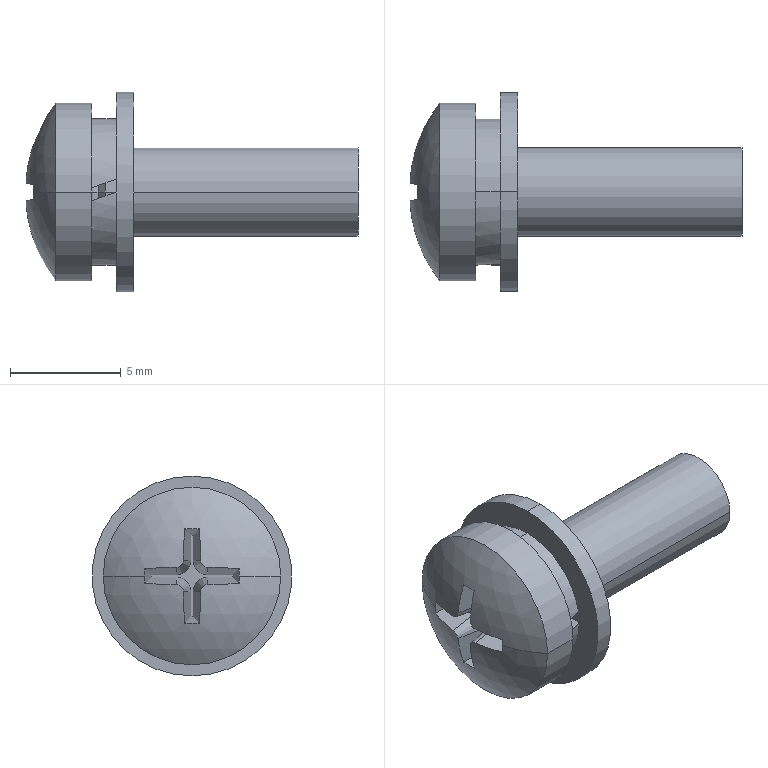Part | SolidWorks | features BaseBody 3 | 3 solids | 45 faces | box 14.964 x 9 x 9 mm | volume 319.965 mm3 | plane 21 | cylinder 14 | cone 6 | sphere 2 | torus 2 | commonest cylinder face diameters 4.4 x3 6.6 x3 4 x2 4.3 x2 8 x2 9 x2
STEP:
#1=CARTESIAN_POINT('',(-133.132,10.87,0.));
#2=VERTEX_POINT('',#1);
#3=CARTESIAN_POINT('',(-133.132,14.87,0.));
#4=VERTEX_POINT('',#3);
#5=CARTESIAN_POINT('',(-133.132,12.87,0.));
#6=DIRECTION('',(-1.,0.,0.));
#7=DIRECTION('',(0.,-1.,0.));
#8=AXIS2_PLACEMENT_3D('',#5,#6,#7);
#9=CIRCLE('',#8,2.);
#10=EDGE_CURVE('',#2,#4,#9,.T.);
#11=ORIENTED_EDGE('',*,*,#10,.T.);
#12=CARTESIAN_POINT('',(-144.532,14.87,0.));
#13=VERTEX_POINT('',#12);
#14=CARTESIAN_POINT('',(-148.132,14.87,0.));
#15=DIRECTION('',(-1.,0.,0.));
#16=VECTOR('',#15,1000.);
#17=LINE('',#14,#16);
#18=EDGE_CURVE('',#4,#13,#17,.T.);
#19=ORIENTED_EDGE('',*,*,#18,.T.);
#20=CARTESIAN_POINT('',(-144.532,10.87,0.));
#21=VERTEX_POINT('',#20);
#22=CARTESIAN_POINT('',(-144.532,12.87,0.));
#23=DIRECTION('',(-1.,0.,0.));
#24=DIRECTION('',(0.,-1.,0.));
#25=AXIS2_PLACEMENT_3D('',#22,#23,#24);
#26=CIRCLE('',#25,2.);
#27=EDGE_CURVE('',#21,#13,#26,.T.);
#28=ORIENTED_EDGE('',*,*,#27,.F.);
#29=CARTESIAN_POINT('',(-148.132,10.87,0.));
#30=DIRECTION('',(-1.,0.,0.));
#31=VECTOR('',#30,1000.);
#32=LINE('',#29,#31);
#33=EDGE_CURVE('',#2,#21,#32,.T.);
#34=ORIENTED_EDGE('',*,*,#33,.F.);
#35=EDGE_LOOP('',(#11,#19,#28,#34));
#36=FACE_OUTER_BOUND('',#35,.T.);
#37=CARTESIAN_POINT('',(-148.132,12.87,0.));
#38=DIRECTION('',(-1.,0.,0.));
#39=DIRECTION('',(0.,-1.,0.));
#40=AXIS2_PLACEMENT_3D('',#37,#38,#39);
#41=CYLINDRICAL_SURFACE('',#40,2.);
#42=ADVANCED_FACE('',(#36),#41,.T.);
#43=CARTESIAN_POINT('',(-146.755,16.87,0.));
#44=VERTEX_POINT('',#43);
#45=CARTESIAN_POINT('',(-146.755,8.87,0.));
#46=VERTEX_POINT('',#45);
#47=CARTESIAN_POINT('',(-146.755,12.87,0.));
#48=DIRECTION('',(-1.,0.,0.));
#49=DIRECTION('',(0.,-1.,0.));
#50=AXIS2_PLACEMENT_3D('',#47,#48,#49);
#51=CIRCLE('',#50,4.);
#52=EDGE_CURVE('',#44,#46,#51,.T.);
#53=ORIENTED_EDGE('',*,*,#52,.T.);
#54=CARTESIAN_POINT('',(-147.771,10.734,0.));
#55=VERTEX_POINT('',#54);
#56=CARTESIAN_POINT('',(-141.632,12.87,0.));
#57=DIRECTION('',(0.,0.,-1.));
#58=DIRECTION('',(0.,1.,0.));
#59=AXIS2_PLACEMENT_3D('',#56,#57,#58);
#60=CIRCLE('',#59,6.5);
#61=EDGE_CURVE('',#46,#55,#60,.T.);
#62=ORIENTED_EDGE('',*,*,#61,.T.);
#63=CARTESIAN_POINT('',(-147.762,10.735,-0.3348));
#64=VERTEX_POINT('',#63);
#65=CARTESIAN_POINT('',(-141.451,11.848,0.));
#66=DIRECTION('',(0.1736,-0.9848,0.));
#67=DIRECTION('',(0.9848,0.1736,0.));
#68=AXIS2_PLACEMENT_3D('',#65,#66,#67);
#69=CIRCLE('',#68,6.417);
#70=EDGE_CURVE('',#55,#64,#69,.T.);
#71=ORIENTED_EDGE('',*,*,#70,.T.);
#72=CARTESIAN_POINT('',(-148.082,12.17,-0.3912));
#73=VERTEX_POINT('',#72);
#74=CARTESIAN_POINT('',(-141.759,12.87,0.7236));
#75=DIRECTION('',(0.1736,0.,-0.9848));
#76=DIRECTION('',(-0.9848,0.,-0.1736));
#77=AXIS2_PLACEMENT_3D('',#74,#75,#76);
#78=CIRCLE('',#77,6.458);
#79=EDGE_CURVE('',#64,#73,#78,.T.);
#80=ORIENTED_EDGE('',*,*,#79,.T.);
#81=CARTESIAN_POINT('',(-148.082,12.479,-0.7));
#82=VERTEX_POINT('',#81);
#83=CARTESIAN_POINT('',(-148.082,12.17,-0.3912));
#84=CARTESIAN_POINT('',(-148.091,12.251,-0.3928));
#85=CARTESIAN_POINT('',(-148.096,12.33,-0.4265));
#86=CARTESIAN_POINT('',(-148.096,12.444,-0.5401));
#87=CARTESIAN_POINT('',(-148.091,12.477,-0.6192));
#88=CARTESIAN_POINT('',(-148.082,12.479,-0.7));
#89=B_SPLINE_CURVE_WITH_KNOTS('',3,(#83,#84,#85,#86,#87,#88),.UNSPECIFIED.,.F.,.F.,(4,2,4),(0.000000198,0.0002406,0.0004811),.UNSPECIFIED.);
#90=EDGE_CURVE('',#73,#82,#89,.T.);
#91=ORIENTED_EDGE('',*,*,#90,.T.);
#92=CARTESIAN_POINT('',(-147.762,12.535,-2.135));
#93=VERTEX_POINT('',#92);
#94=CARTESIAN_POINT('',(-141.759,13.594,0.));
#95=DIRECTION('',(0.1736,-0.9848,0.));
#96=DIRECTION('',(0.9848,0.1736,0.));
#97=AXIS2_PLACEMENT_3D('',#94,#95,#96);
#98=CIRCLE('',#97,6.458);
#99=EDGE_CURVE('',#82,#93,#98,.T.);
#100=ORIENTED_EDGE('',*,*,#99,.T.);
#101=CARTESIAN_POINT('',(-147.762,13.205,-2.135));
#102=VERTEX_POINT('',#101);
#103=CARTESIAN_POINT('',(-141.451,12.87,-1.022));
#104=DIRECTION('',(0.1736,0.,-0.9848));
#105=DIRECTION('',(-0.9848,0.,-0.1736));
#106=AXIS2_PLACEMENT_3D('',#103,#104,#105);
#107=CIRCLE('',#106,6.417);
#108=EDGE_CURVE('',#93,#102,#107,.T.);
#109=ORIENTED_EDGE('',*,*,#108,.T.);
#110=CARTESIAN_POINT('',(-148.082,13.261,-0.7));
#111=VERTEX_POINT('',#110);
#112=CARTESIAN_POINT('',(-141.759,12.147,0.));
#113=DIRECTION('',(0.1736,0.9848,0.));
#114=DIRECTION('',(-0.9848,0.1736,0.));
#115=AXIS2_PLACEMENT_3D('',#112,#113,#114);
#116=CIRCLE('',#115,6.458);
#117=EDGE_CURVE('',#102,#111,#116,.T.);
#118=ORIENTED_EDGE('',*,*,#117,.T.);
#119=CARTESIAN_POINT('',(-148.082,13.57,-0.3912));
#120=VERTEX_POINT('',#119);
#121=CARTESIAN_POINT('',(-148.082,13.261,-0.7));
#122=CARTESIAN_POINT('',(-148.091,13.263,-0.6192));
#123=CARTESIAN_POINT('',(-148.096,13.297,-0.5403));
#124=CARTESIAN_POINT('',(-148.096,13.41,-0.4266));
#125=CARTESIAN_POINT('',(-148.091,13.489,-0.3928));
#126=CARTESIAN_POINT('',(-148.082,13.57,-0.3912));
#127=B_SPLINE_CURVE_WITH_KNOTS('',3,(#121,#122,#123,#124,#125,#126),.UNSPECIFIED.,.F.,.F.,(4,2,4),(0.000000198,0.0002406,0.0004811),.UNSPECIFIED.);
#128=EDGE_CURVE('',#111,#120,#127,.T.);
#129=ORIENTED_EDGE('',*,*,#128,.T.);
#130=CARTESIAN_POINT('',(-147.762,15.005,-0.3348));
#131=VERTEX_POINT('',#130);
#132=CARTESIAN_POINT('',(-141.759,12.87,0.7236));
#133=DIRECTION('',(0.1736,0.,-0.9848));
#134=DIRECTION('',(-0.9848,0.,-0.1736));
#135=AXIS2_PLACEMENT_3D('',#132,#133,#134);
#136=CIRCLE('',#135,6.458);
#137=EDGE_CURVE('',#120,#131,#136,.T.);
#138=ORIENTED_EDGE('',*,*,#137,.T.);
#139=CARTESIAN_POINT('',(-147.771,15.007,0.));
#140=VERTEX_POINT('',#139);
#141=CARTESIAN_POINT('',(-141.451,13.892,0.));
#142=DIRECTION('',(0.1736,0.9848,0.));
#143=DIRECTION('',(-0.9848,0.1736,0.));
#144=AXIS2_PLACEMENT_3D('',#141,#142,#143);
#145=CIRCLE('',#144,6.417);
#146=EDGE_CURVE('',#131,#140,#145,.T.);
#147=ORIENTED_EDGE('',*,*,#146,.T.);
#148=CARTESIAN_POINT('',(-141.632,12.87,0.));
#149=DIRECTION('',(0.,0.,1.));
#150=DIRECTION('',(1.,0.,0.));
#151=AXIS2_PLACEMENT_3D('',#148,#149,#150);
#152=CIRCLE('',#151,6.5);
#153=EDGE_CURVE('',#44,#140,#152,.T.);
#154=ORIENTED_EDGE('',*,*,#153,.F.);
#155=EDGE_LOOP('',(#53,#62,#71,#80,#91,#100,#109,#118,#129,#138,#147,#154));
#156=FACE_OUTER_BOUND('',#155,.T.);
#157=CARTESIAN_POINT('',(-141.632,12.87,0.));
#158=DIRECTION('',(0.,0.,-1.));
#159=DIRECTION('',(0.,1.,0.));
#160=AXIS2_PLACEMENT_3D('',#157,#158,#159);
#161=SPHERICAL_SURFACE('',#160,6.5);
#162=ADVANCED_FACE('',(#156),#161,.T.);
#163=CARTESIAN_POINT('',(-145.132,8.87,0.));
#164=VERTEX_POINT('',#163);
#165=CARTESIAN_POINT('',(-145.132,16.87,0.));
#166=VERTEX_POINT('',#165);
#167=CARTESIAN_POINT('',(-145.132,12.87,0.));
#168=DIRECTION('',(-1.,0.,0.));
#169=DIRECTION('',(0.,-1.,0.));
#170=AXIS2_PLACEMENT_3D('',#167,#168,#169);
#171=CIRCLE('',#170,4.);
#172=EDGE_CURVE('',#164,#166,#171,.T.);
#173=ORIENTED_EDGE('',*,*,#172,.T.);
#174=CARTESIAN_POINT('',(-148.132,16.87,0.));
#175=DIRECTION('',(-1.,0.,0.));
#176=VECTOR('',#175,1000.);
#177=LINE('',#174,#176);
#178=EDGE_CURVE('',#166,#44,#177,.T.);
#179=ORIENTED_EDGE('',*,*,#178,.T.);
#180=CARTESIAN_POINT('',(-146.755,12.87,0.));
#181=DIRECTION('',(-1.,0.,0.));
#182=DIRECTION('',(0.,-1.,0.));
#183=AXIS2_PLACEMENT_3D('',#180,#181,#182);
#184=CIRCLE('',#183,4.);
#185=EDGE_CURVE('',#46,#44,#184,.T.);
#186=ORIENTED_EDGE('',*,*,#185,.F.);
#187=CARTESIAN_POINT('',(-148.132,8.87,0.));
#188=DIRECTION('',(-1.,0.,0.));
#189=VECTOR('',#188,1000.);
#190=LINE('',#187,#189);
#191=EDGE_CURVE('',#164,#46,#190,.T.);
#192=ORIENTED_EDGE('',*,*,#191,.F.);
#193=EDGE_LOOP('',(#173,#179,#186,#192));
#194=FACE_OUTER_BOUND('',#193,.T.);
#195=CARTESIAN_POINT('',(-148.132,12.87,0.));
#196=DIRECTION('',(-1.,0.,0.));
#197=DIRECTION('',(0.,-1.,0.));
#198=AXIS2_PLACEMENT_3D('',#195,#196,#197);
#199=CYLINDRICAL_SURFACE('',#198,4.);
#200=ADVANCED_FACE('',(#194),#199,.T.);
#201=CARTESIAN_POINT('',(-145.132,14.87,0.));
#202=VERTEX_POINT('',#201);
#203=CARTESIAN_POINT('',(-145.132,10.87,0.));
#204=VERTEX_POINT('',#203);
#205=CARTESIAN_POINT('',(-145.132,12.87,0.));
#206=DIRECTION('',(-1.,0.,0.));
#207=DIRECTION('',(0.,-1.,0.));
#208=AXIS2_PLACEMENT_3D('',#205,#206,#207);
#209=CIRCLE('',#208,2.);
#210=EDGE_CURVE('',#202,#204,#209,.T.);
#211=ORIENTED_EDGE('',*,*,#210,.F.);
#212=CARTESIAN_POINT('',(-144.832,14.57,0.));
#213=VERTEX_POINT('',#212);
#214=CARTESIAN_POINT('',(-144.832,14.87,0.));
#215=DIRECTION('',(0.,0.,1.));
#216=DIRECTION('',(0.,-1.,0.));
#217=AXIS2_PLACEMENT_3D('',#214,#215,#216);
#218=CIRCLE('',#217,0.3);
#219=EDGE_CURVE('',#202,#213,#218,.T.);
#220=ORIENTED_EDGE('',*,*,#219,.T.);
#221=CARTESIAN_POINT('',(-144.832,11.17,0.));
#222=VERTEX_POINT('',#221);
#223=CARTESIAN_POINT('',(-144.832,12.87,0.));
#224=DIRECTION('',(-1.,0.,0.));
#225=DIRECTION('',(0.,-1.,0.));
#226=AXIS2_PLACEMENT_3D('',#223,#224,#225);
#227=CIRCLE('',#226,1.7);
#228=EDGE_CURVE('',#213,#222,#227,.T.);
#229=ORIENTED_EDGE('',*,*,#228,.T.);
#230=CARTESIAN_POINT('',(-144.832,10.87,0.));
#231=DIRECTION('',(0.,0.,-1.));
#232=DIRECTION('',(-1.,0.,0.));
#233=AXIS2_PLACEMENT_3D('',#230,#231,#232);
#234=CIRCLE('',#233,0.3);
#235=EDGE_CURVE('',#204,#222,#234,.T.);
#236=ORIENTED_EDGE('',*,*,#235,.F.);
#237=EDGE_LOOP('',(#211,#220,#229,#236));
#238=FACE_OUTER_BOUND('',#237,.T.);
#239=CARTESIAN_POINT('',(-144.832,12.87,0.));
#240=DIRECTION('',(-1.,0.,0.));
#241=DIRECTION('',(0.,-1.,0.));
#242=AXIS2_PLACEMENT_3D('',#239,#240,#241);
#243=TOROIDAL_SURFACE('',#242,2.,0.3);
#244=ADVANCED_FACE('',(#238),#243,.F.);
#245=CARTESIAN_POINT('',(-144.832,12.87,0.));
#246=DIRECTION('',(-1.,0.,0.));
#247=DIRECTION('',(0.,-1.,0.));
#248=AXIS2_PLACEMENT_3D('',#245,#246,#247);
#249=CIRCLE('',#248,1.7);
#250=EDGE_CURVE('',#222,#213,#249,.T.);
#251=ORIENTED_EDGE('',*,*,#250,.F.);
#252=CARTESIAN_POINT('',(-144.832,11.17,0.));
#253=DIRECTION('',(0.7071,-0.7071,0.));
#254=VECTOR('',#253,1000.);
#255=LINE('',#252,#254);
#256=EDGE_CURVE('',#222,#21,#255,.T.);
#257=ORIENTED_EDGE('',*,*,#256,.T.);
#258=ORIENTED_EDGE('',*,*,#27,.T.);
#259=CARTESIAN_POINT('',(-144.832,14.57,0.));
#260=DIRECTION('',(0.7071,0.7071,0.));
#261=VECTOR('',#260,1000.);
#262=LINE('',#259,#261);
#263=EDGE_CURVE('',#213,#13,#262,.T.);
#264=ORIENTED_EDGE('',*,*,#263,.F.);
#265=EDGE_LOOP('',(#251,#257,#258,#264));
#266=FACE_OUTER_BOUND('',#265,.T.);
#267=CARTESIAN_POINT('',(-144.832,12.87,0.));
#268=DIRECTION('',(1.,0.,0.));
#269=DIRECTION('',(0.,1.,0.));
#270=AXIS2_PLACEMENT_3D('',#267,#268,#269);
#271=CONICAL_SURFACE('',#270,1.7,0.7854);
#272=ADVANCED_FACE('',(#266),#271,.T.);
#273=ORIENTED_EDGE('',*,*,#256,.F.);
#274=ORIENTED_EDGE('',*,*,#228,.F.);
#275=ORIENTED_EDGE('',*,*,#263,.T.);
#276=CARTESIAN_POINT('',(-144.532,12.87,0.));
#277=DIRECTION('',(-1.,0.,0.));
#278=DIRECTION('',(0.,-1.,0.));
#279=AXIS2_PLACEMENT_3D('',#276,#277,#278);
#280=CIRCLE('',#279,2.);
#281=EDGE_CURVE('',#13,#21,#280,.T.);
#282=ORIENTED_EDGE('',*,*,#281,.T.);
#283=EDGE_LOOP('',(#273,#274,#275,#282));
#284=FACE_OUTER_BOUND('',#283,.T.);
#285=CARTESIAN_POINT('',(-144.832,12.87,0.));
#286=DIRECTION('',(1.,0.,0.));
#287=DIRECTION('',(0.,1.,0.));
#288=AXIS2_PLACEMENT_3D('',#285,#286,#287);
#289=CONICAL_SURFACE('',#288,1.7,0.7854);
#290=ADVANCED_FACE('',(#284),#289,.T.);
#291=ORIENTED_EDGE('',*,*,#219,.F.);
#292=CARTESIAN_POINT('',(-145.132,12.87,0.));
#293=DIRECTION('',(-1.,0.,0.));
#294=DIRECTION('',(0.,-1.,0.));
#295=AXIS2_PLACEMENT_3D('',#292,#293,#294);
#296=CIRCLE('',#295,2.);
#297=EDGE_CURVE('',#204,#202,#296,.T.);
#298=ORIENTED_EDGE('',*,*,#297,.F.);
#299=ORIENTED_EDGE('',*,*,#235,.T.);
#300=ORIENTED_EDGE('',*,*,#250,.T.);
#301=EDGE_LOOP('',(#291,#298,#299,#300));
#302=FACE_OUTER_BOUND('',#301,.T.);
#303=CARTESIAN_POINT('',(-144.832,12.87,0.));
#304=DIRECTION('',(-1.,0.,0.));
#305=DIRECTION('',(0.,-1.,0.));
#306=AXIS2_PLACEMENT_3D('',#303,#304,#305);
#307=TOROIDAL_SURFACE('',#306,2.,0.3);
#308=ADVANCED_FACE('',(#302),#307,.F.);
#309=ORIENTED_EDGE('',*,*,#172,.F.);
#310=CARTESIAN_POINT('',(-145.132,12.87,0.));
#311=DIRECTION('',(-1.,0.,0.));
#312=DIRECTION('',(0.,-1.,0.));
#313=AXIS2_PLACEMENT_3D('',#310,#311,#312);
#314=CIRCLE('',#313,4.);
#315=EDGE_CURVE('',#166,#164,#314,.T.);
#316=ORIENTED_EDGE('',*,*,#315,.F.);
#317=EDGE_LOOP('',(#309,#316));
#318=FACE_OUTER_BOUND('',#317,.T.);
#319=ORIENTED_EDGE('',*,*,#297,.T.);
#320=ORIENTED_EDGE('',*,*,#210,.T.);
#321=EDGE_LOOP('',(#319,#320));
#322=FACE_BOUND('',#321,.T.);
#323=CARTESIAN_POINT('',(-145.132,12.87,0.));
#324=DIRECTION('',(-1.,0.,0.));
#325=DIRECTION('',(0.,-1.,0.));
#326=AXIS2_PLACEMENT_3D('',#323,#324,#325);
#327=PLANE('',#326);
#328=ADVANCED_FACE('',(#318,#322),#327,.F.);
#329=ORIENTED_EDGE('',*,*,#178,.F.);
#330=ORIENTED_EDGE('',*,*,#315,.T.);
#331=ORIENTED_EDGE('',*,*,#191,.T.);
#332=ORIENTED_EDGE('',*,*,#52,.F.);
#333=EDGE_LOOP('',(#329,#330,#331,#332));
#334=FACE_OUTER_BOUND('',#333,.T.);
#335=CARTESIAN_POINT('',(-148.132,12.87,0.));
#336=DIRECTION('',(-1.,0.,0.));
#337=DIRECTION('',(0.,-1.,0.));
#338=AXIS2_PLACEMENT_3D('',#335,#336,#337);
#339=CYLINDRICAL_SURFACE('',#338,4.);
#340=ADVANCED_FACE('',(#334),#339,.T.);
#341=ORIENTED_EDGE('',*,*,#61,.F.);
#342=ORIENTED_EDGE('',*,*,#185,.T.);
#343=ORIENTED_EDGE('',*,*,#153,.T.);
#344=CARTESIAN_POINT('',(-147.762,15.005,0.3348));
#345=VERTEX_POINT('',#344);
#346=CARTESIAN_POINT('',(-141.451,13.892,0.));
#347=DIRECTION('',(0.1736,0.9848,0.));
#348=DIRECTION('',(-0.9848,0.1736,0.));
#349=AXIS2_PLACEMENT_3D('',#346,#347,#348);
#350=CIRCLE('',#349,6.417);
#351=EDGE_CURVE('',#140,#345,#350,.T.);
#352=ORIENTED_EDGE('',*,*,#351,.T.);
#353=CARTESIAN_POINT('',(-148.082,13.57,0.3912));
#354=VERTEX_POINT('',#353);
#355=CARTESIAN_POINT('',(-141.759,12.87,-0.7236));
#356=DIRECTION('',(0.1736,0.,0.9848));
#357=DIRECTION('',(0.9848,0.,-0.1736));
#358=AXIS2_PLACEMENT_3D('',#355,#356,#357);
#359=CIRCLE('',#358,6.458);
#360=EDGE_CURVE('',#345,#354,#359,.T.);
#361=ORIENTED_EDGE('',*,*,#360,.T.);
#362=CARTESIAN_POINT('',(-148.082,13.261,0.7));
#363=VERTEX_POINT('',#362);
#364=CARTESIAN_POINT('',(-148.082,13.57,0.3912));
#365=CARTESIAN_POINT('',(-148.091,13.489,0.3928));
#366=CARTESIAN_POINT('',(-148.096,13.41,0.4265));
#367=CARTESIAN_POINT('',(-148.096,13.297,0.5401));
#368=CARTESIAN_POINT('',(-148.091,13.263,0.6192));
#369=CARTESIAN_POINT('',(-148.082,13.261,0.7));
#370=B_SPLINE_CURVE_WITH_KNOTS('',3,(#364,#365,#366,#367,#368,#369),.UNSPECIFIED.,.F.,.F.,(4,2,4),(0.000000198,0.0002406,0.0004811),.UNSPECIFIED.);
#371=EDGE_CURVE('',#354,#363,#370,.T.);
#372=ORIENTED_EDGE('',*,*,#371,.T.);
#373=CARTESIAN_POINT('',(-147.762,13.205,2.135));
#374=VERTEX_POINT('',#373);
#375=CARTESIAN_POINT('',(-141.759,12.147,0.));
#376=DIRECTION('',(0.1736,0.9848,0.));
#377=DIRECTION('',(-0.9848,0.1736,0.));
#378=AXIS2_PLACEMENT_3D('',#375,#376,#377);
#379=CIRCLE('',#378,6.458);
#380=EDGE_CURVE('',#363,#374,#379,.T.);
#381=ORIENTED_EDGE('',*,*,#380,.T.);
#382=CARTESIAN_POINT('',(-147.762,12.535,2.135));
#383=VERTEX_POINT('',#382);
#384=CARTESIAN_POINT('',(-141.451,12.87,1.022));
#385=DIRECTION('',(0.1736,0.,0.9848));
#386=DIRECTION('',(0.9848,0.,-0.1736));
#387=AXIS2_PLACEMENT_3D('',#384,#385,#386);
#388=CIRCLE('',#387,6.417);
#389=EDGE_CURVE('',#374,#383,#388,.T.);
#390=ORIENTED_EDGE('',*,*,#389,.T.);
#391=CARTESIAN_POINT('',(-148.082,12.479,0.7));
#392=VERTEX_POINT('',#391);
#393=CARTESIAN_POINT('',(-141.759,13.594,0.));
#394=DIRECTION('',(0.1736,-0.9848,0.));
#395=DIRECTION('',(0.9848,0.1736,0.));
#396=AXIS2_PLACEMENT_3D('',#393,#394,#395);
#397=CIRCLE('',#396,6.458);
#398=EDGE_CURVE('',#383,#392,#397,.T.);
#399=ORIENTED_EDGE('',*,*,#398,.T.);
#400=CARTESIAN_POINT('',(-148.082,12.17,0.3912));
#401=VERTEX_POINT('',#400);
#402=CARTESIAN_POINT('',(-148.082,12.479,0.7));
#403=CARTESIAN_POINT('',(-148.091,12.477,0.6192));
#404=CARTESIAN_POINT('',(-148.096,12.444,0.5403));
#405=CARTESIAN_POINT('',(-148.096,12.33,0.4266));
#406=CARTESIAN_POINT('',(-148.091,12.251,0.3928));
#407=CARTESIAN_POINT('',(-148.082,12.17,0.3912));
#408=B_SPLINE_CURVE_WITH_KNOTS('',3,(#402,#403,#404,#405,#406,#407),.UNSPECIFIED.,.F.,.F.,(4,2,4),(0.000000198,0.0002406,0.0004811),.UNSPECIFIED.);
#409=EDGE_CURVE('',#392,#401,#408,.T.);
#410=ORIENTED_EDGE('',*,*,#409,.T.);
#411=CARTESIAN_POINT('',(-147.762,10.735,0.3348));
#412=VERTEX_POINT('',#411);
#413=CARTESIAN_POINT('',(-141.759,12.87,-0.7236));
#414=DIRECTION('',(0.1736,0.,0.9848));
#415=DIRECTION('',(0.9848,0.,-0.1736));
#416=AXIS2_PLACEMENT_3D('',#413,#414,#415);
#417=CIRCLE('',#416,6.458);
#418=EDGE_CURVE('',#401,#412,#417,.T.);
#419=ORIENTED_EDGE('',*,*,#418,.T.);
#420=CARTESIAN_POINT('',(-141.451,11.848,0.));
#421=DIRECTION('',(0.1736,-0.9848,0.));
#422=DIRECTION('',(0.9848,0.1736,0.));
#423=AXIS2_PLACEMENT_3D('',#420,#421,#422);
#424=CIRCLE('',#423,6.417);
#425=EDGE_CURVE('',#412,#55,#424,.T.);
#426=ORIENTED_EDGE('',*,*,#425,.T.);
#427=EDGE_LOOP('',(#341,#342,#343,#352,#361,#372,#381,#390,#399,#410,#419,#426));
#428=FACE_OUTER_BOUND('',#427,.T.);
#429=CARTESIAN_POINT('',(-141.632,12.87,0.));
#430=DIRECTION('',(0.,0.,-1.));
#431=DIRECTION('',(0.,1.,0.));
#432=AXIS2_PLACEMENT_3D('',#429,#430,#431);
#433=SPHERICAL_SURFACE('',#432,6.5);
#434=ADVANCED_FACE('',(#428),#433,.T.);
#435=ORIENTED_EDGE('',*,*,#10,.F.);
#436=CARTESIAN_POINT('',(-133.132,12.87,0.));
#437=DIRECTION('',(-1.,0.,0.));
#438=DIRECTION('',(0.,-1.,0.));
#439=AXIS2_PLACEMENT_3D('',#436,#437,#438);
#440=CIRCLE('',#439,2.);
#441=EDGE_CURVE('',#4,#2,#440,.T.);
#442=ORIENTED_EDGE('',*,*,#441,.F.);
#443=EDGE_LOOP('',(#435,#442));
#444=FACE_OUTER_BOUND('',#443,.T.);
#445=CARTESIAN_POINT('',(-133.132,12.87,0.));
#446=DIRECTION('',(1.,0.,0.));
#447=DIRECTION('',(0.,1.,0.));
#448=AXIS2_PLACEMENT_3D('',#445,#446,#447);
#449=PLANE('',#448);
#450=ADVANCED_FACE('',(#444),#449,.T.);
#451=ORIENTED_EDGE('',*,*,#18,.F.);
#452=ORIENTED_EDGE('',*,*,#441,.T.);
#453=ORIENTED_EDGE('',*,*,#33,.T.);
#454=ORIENTED_EDGE('',*,*,#281,.F.);
#455=EDGE_LOOP('',(#451,#452,#453,#454));
#456=FACE_OUTER_BOUND('',#455,.T.);
#457=CARTESIAN_POINT('',(-148.132,12.87,0.));
#458=DIRECTION('',(-1.,0.,0.));
#459=DIRECTION('',(0.,-1.,0.));
#460=AXIS2_PLACEMENT_3D('',#457,#458,#459);
#461=CYLINDRICAL_SURFACE('',#460,2.);
#462=ADVANCED_FACE('',(#456),#461,.T.);
#463=CARTESIAN_POINT('',(-146.132,11.023,-0.04735));
#464=VERTEX_POINT('',#463);
#465=CARTESIAN_POINT('',(-147.883,10.714,-0.3561));
#466=DIRECTION('',(-0.9703,-0.1711,-0.1711));
#467=VECTOR('',#466,1000.);
#468=LINE('',#465,#467);
#469=EDGE_CURVE('',#464,#64,#468,.T.);
#470=ORIENTED_EDGE('',*,*,#469,.F.);
#471=CARTESIAN_POINT('',(-146.132,12.17,-0.04735));
#472=VERTEX_POINT('',#471);
#473=CARTESIAN_POINT('',(-146.132,12.17,-0.04735));
#474=DIRECTION('',(0.,-1.,0.));
#475=VECTOR('',#474,1000.);
#476=LINE('',#473,#475);
#477=EDGE_CURVE('',#472,#464,#476,.T.);
#478=ORIENTED_EDGE('',*,*,#477,.F.);
#479=CARTESIAN_POINT('',(-148.132,12.17,-0.4));
#480=DIRECTION('',(-0.9848,0.,-0.1736));
#481=VECTOR('',#480,1000.);
#482=LINE('',#479,#481);
#483=EDGE_CURVE('',#472,#73,#482,.T.);
#484=ORIENTED_EDGE('',*,*,#483,.T.);
#485=ORIENTED_EDGE('',*,*,#79,.F.);
#486=EDGE_LOOP('',(#470,#478,#484,#485));
#487=FACE_OUTER_BOUND('',#486,.T.);
#488=CARTESIAN_POINT('',(-148.132,12.17,-0.4));
#489=DIRECTION('',(0.1736,0.,-0.9848));
#490=DIRECTION('',(-0.9848,0.,-0.1736));
#491=AXIS2_PLACEMENT_3D('',#488,#489,#490);
#492=PLANE('',#491);
#493=ADVANCED_FACE('',(#487),#492,.F.);
#494=ORIENTED_EDGE('',*,*,#483,.F.);
#495=CARTESIAN_POINT('',(-146.132,12.823,-0.7));
#496=VERTEX_POINT('',#495);
#497=CARTESIAN_POINT('',(-146.132,12.17,-0.7));
#498=DIRECTION('',(1.,0.,0.));
#499=DIRECTION('',(0.,0.,1.));
#500=AXIS2_PLACEMENT_3D('',#497,#498,#499);
#501=CIRCLE('',#500,0.6527);
#502=EDGE_CURVE('',#496,#472,#501,.T.);
#503=ORIENTED_EDGE('',*,*,#502,.F.);
#504=CARTESIAN_POINT('',(-148.132,12.47,-0.7));
#505=DIRECTION('',(-0.9848,-0.1736,0.));
#506=VECTOR('',#505,1000.);
#507=LINE('',#504,#506);
#508=EDGE_CURVE('',#496,#82,#507,.T.);
#509=ORIENTED_EDGE('',*,*,#508,.T.);
#510=ORIENTED_EDGE('',*,*,#90,.F.);
#511=EDGE_LOOP('',(#494,#503,#509,#510));
#512=FACE_OUTER_BOUND('',#511,.T.);
#513=CARTESIAN_POINT('',(-148.132,12.17,-0.7));
#514=DIRECTION('',(1.,0.,0.));
#515=DIRECTION('',(0.,0.,-1.));
#516=AXIS2_PLACEMENT_3D('',#513,#514,#515);
#517=CONICAL_SURFACE('',#516,0.3,0.1745);
#518=ADVANCED_FACE('',(#512),#517,.T.);
#519=ORIENTED_EDGE('',*,*,#508,.F.);
#520=CARTESIAN_POINT('',(-146.132,12.823,-1.847));
#521=VERTEX_POINT('',#520);
#522=CARTESIAN_POINT('',(-146.132,12.823,0.7));
#523=DIRECTION('',(0.,0.,1.));
#524=VECTOR('',#523,1000.);
#525=LINE('',#522,#524);
#526=EDGE_CURVE('',#521,#496,#525,.T.);
#527=ORIENTED_EDGE('',*,*,#526,.F.);
#528=CARTESIAN_POINT('',(-148.132,12.47,-2.2));
#529=DIRECTION('',(-0.9703,-0.1711,-0.1711));
#530=VECTOR('',#529,1000.);
#531=LINE('',#528,#530);
#532=EDGE_CURVE('',#521,#93,#531,.T.);
#533=ORIENTED_EDGE('',*,*,#532,.T.);
#534=ORIENTED_EDGE('',*,*,#99,.F.);
#535=EDGE_LOOP('',(#519,#527,#533,#534));
#536=FACE_OUTER_BOUND('',#535,.T.);
#537=CARTESIAN_POINT('',(-148.132,12.47,-2.2));
#538=DIRECTION('',(0.1736,-0.9848,0.));
#539=DIRECTION('',(0.9848,0.1736,0.));
#540=AXIS2_PLACEMENT_3D('',#537,#538,#539);
#541=PLANE('',#540);
#542=ADVANCED_FACE('',(#536),#541,.F.);
#543=ORIENTED_EDGE('',*,*,#532,.F.);
#544=CARTESIAN_POINT('',(-146.132,12.918,-1.847));
#545=VERTEX_POINT('',#544);
#546=CARTESIAN_POINT('',(-146.132,12.17,-1.847));
#547=DIRECTION('',(0.,-1.,0.));
#548=VECTOR('',#547,1000.);
#549=LINE('',#546,#548);
#550=EDGE_CURVE('',#545,#521,#549,.T.);
#551=ORIENTED_EDGE('',*,*,#550,.F.);
#552=CARTESIAN_POINT('',(-148.132,13.27,-2.2));
#553=DIRECTION('',(-0.9703,0.1711,-0.1711));
#554=VECTOR('',#553,1000.);
#555=LINE('',#552,#554);
#556=EDGE_CURVE('',#545,#102,#555,.T.);
#557=ORIENTED_EDGE('',*,*,#556,.T.);
#558=ORIENTED_EDGE('',*,*,#108,.F.);
#559=EDGE_LOOP('',(#543,#551,#557,#558));
#560=FACE_OUTER_BOUND('',#559,.T.);
#561=CARTESIAN_POINT('',(-148.132,12.47,-2.2));
#562=DIRECTION('',(0.1736,0.,-0.9848));
#563=DIRECTION('',(-0.9848,0.,-0.1736));
#564=AXIS2_PLACEMENT_3D('',#561,#562,#563);
#565=PLANE('',#564);
#566=ADVANCED_FACE('',(#560),#565,.F.);
#567=ORIENTED_EDGE('',*,*,#556,.F.);
#568=CARTESIAN_POINT('',(-146.132,12.918,-0.7));
#569=VERTEX_POINT('',#568);
#570=CARTESIAN_POINT('',(-146.132,12.918,0.7));
#571=DIRECTION('',(0.,0.,-1.));
#572=VECTOR('',#571,1000.);
#573=LINE('',#570,#572);
#574=EDGE_CURVE('',#569,#545,#573,.T.);
#575=ORIENTED_EDGE('',*,*,#574,.F.);
#576=CARTESIAN_POINT('',(-148.132,13.27,-0.7));
#577=DIRECTION('',(-0.9848,0.1736,0.));
#578=VECTOR('',#577,1000.);
#579=LINE('',#576,#578);
#580=EDGE_CURVE('',#569,#111,#579,.T.);
#581=ORIENTED_EDGE('',*,*,#580,.T.);
#582=ORIENTED_EDGE('',*,*,#117,.F.);
#583=EDGE_LOOP('',(#567,#575,#581,#582));
#584=FACE_OUTER_BOUND('',#583,.T.);
#585=CARTESIAN_POINT('',(-148.132,13.27,-2.2));
#586=DIRECTION('',(0.1736,0.9848,0.));
#587=DIRECTION('',(-0.9848,0.1736,0.));
#588=AXIS2_PLACEMENT_3D('',#585,#586,#587);
#589=PLANE('',#588);
#590=ADVANCED_FACE('',(#584),#589,.F.);
#591=ORIENTED_EDGE('',*,*,#580,.F.);
#592=CARTESIAN_POINT('',(-146.132,13.57,-0.04735));
#593=VERTEX_POINT('',#592);
#594=CARTESIAN_POINT('',(-146.132,13.57,-0.7));
#595=DIRECTION('',(1.,0.,0.));
#596=DIRECTION('',(0.,0.,1.));
#597=AXIS2_PLACEMENT_3D('',#594,#595,#596);
#598=CIRCLE('',#597,0.6527);
#599=EDGE_CURVE('',#593,#569,#598,.T.);
#600=ORIENTED_EDGE('',*,*,#599,.F.);
#601=CARTESIAN_POINT('',(-148.132,13.57,-0.4));
#602=DIRECTION('',(-0.9848,0.,-0.1736));
#603=VECTOR('',#602,1000.);
#604=LINE('',#601,#603);
#605=EDGE_CURVE('',#593,#120,#604,.T.);
#606=ORIENTED_EDGE('',*,*,#605,.T.);
#607=ORIENTED_EDGE('',*,*,#128,.F.);
#608=EDGE_LOOP('',(#591,#600,#606,#607));
#609=FACE_OUTER_BOUND('',#608,.T.);
#610=CARTESIAN_POINT('',(-148.132,13.57,-0.7));
#611=DIRECTION('',(1.,0.,0.));
#612=DIRECTION('',(0.,0.,1.));
#613=AXIS2_PLACEMENT_3D('',#610,#611,#612);
#614=CONICAL_SURFACE('',#613,0.3,0.1745);
#615=ADVANCED_FACE('',(#609),#614,.T.);
#616=ORIENTED_EDGE('',*,*,#605,.F.);
#617=CARTESIAN_POINT('',(-146.132,14.718,-0.04735));
#618=VERTEX_POINT('',#617);
#619=CARTESIAN_POINT('',(-146.132,12.17,-0.04735));
#620=DIRECTION('',(0.,-1.,0.));
#621=VECTOR('',#620,1000.);
#622=LINE('',#619,#621);
#623=EDGE_CURVE('',#618,#593,#622,.T.);
#624=ORIENTED_EDGE('',*,*,#623,.F.);
#625=CARTESIAN_POINT('',(-147.999,15.047,-0.3766));
#626=DIRECTION('',(-0.9703,0.1711,-0.1711));
#627=VECTOR('',#626,1000.);
#628=LINE('',#625,#627);
#629=EDGE_CURVE('',#618,#131,#628,.T.);
#630=ORIENTED_EDGE('',*,*,#629,.T.);
#631=ORIENTED_EDGE('',*,*,#137,.F.);
#632=EDGE_LOOP('',(#616,#624,#630,#631));
#633=FACE_OUTER_BOUND('',#632,.T.);
#634=CARTESIAN_POINT('',(-148.132,15.07,-0.4));
#635=DIRECTION('',(0.1736,0.,-0.9848));
#636=DIRECTION('',(-0.9848,0.,-0.1736));
#637=AXIS2_PLACEMENT_3D('',#634,#635,#636);
#638=PLANE('',#637);
#639=ADVANCED_FACE('',(#633),#638,.F.);
#640=ORIENTED_EDGE('',*,*,#629,.F.);
#641=CARTESIAN_POINT('',(-146.132,14.718,0.04735));
#642=VERTEX_POINT('',#641);
#643=CARTESIAN_POINT('',(-146.132,14.718,0.7));
#644=DIRECTION('',(0.,0.,-1.));
#645=VECTOR('',#644,1000.);
#646=LINE('',#643,#645);
#647=EDGE_CURVE('',#642,#618,#646,.T.);
#648=ORIENTED_EDGE('',*,*,#647,.F.);
#649=CARTESIAN_POINT('',(-147.883,15.026,0.3561));
#650=DIRECTION('',(-0.9703,0.1711,0.1711));
#651=VECTOR('',#650,1000.);
#652=LINE('',#649,#651);
#653=EDGE_CURVE('',#642,#345,#652,.T.);
#654=ORIENTED_EDGE('',*,*,#653,.T.);
#655=ORIENTED_EDGE('',*,*,#351,.F.);
#656=ORIENTED_EDGE('',*,*,#146,.F.);
#657=EDGE_LOOP('',(#640,#648,#654,#655,#656));
#658=FACE_OUTER_BOUND('',#657,.T.);
#659=CARTESIAN_POINT('',(-148.132,15.07,0.4));
#660=DIRECTION('',(0.1736,0.9848,0.));
#661=DIRECTION('',(-0.9848,0.1736,0.));
#662=AXIS2_PLACEMENT_3D('',#659,#660,#661);
#663=PLANE('',#662);
#664=ADVANCED_FACE('',(#658),#663,.F.);
#665=ORIENTED_EDGE('',*,*,#653,.F.);
#666=CARTESIAN_POINT('',(-146.132,13.57,0.04735));
#667=VERTEX_POINT('',#666);
#668=CARTESIAN_POINT('',(-146.132,12.17,0.04735));
#669=DIRECTION('',(0.,1.,0.));
#670=VECTOR('',#669,1000.);
#671=LINE('',#668,#670);
#672=EDGE_CURVE('',#667,#642,#671,.T.);
#673=ORIENTED_EDGE('',*,*,#672,.F.);
#674=CARTESIAN_POINT('',(-148.132,13.57,0.4));
#675=DIRECTION('',(-0.9848,0.,0.1736));
#676=VECTOR('',#675,1000.);
#677=LINE('',#674,#676);
#678=EDGE_CURVE('',#667,#354,#677,.T.);
#679=ORIENTED_EDGE('',*,*,#678,.T.);
#680=ORIENTED_EDGE('',*,*,#360,.F.);
#681=EDGE_LOOP('',(#665,#673,#679,#680));
#682=FACE_OUTER_BOUND('',#681,.T.);
#683=CARTESIAN_POINT('',(-148.132,13.57,0.4));
#684=DIRECTION('',(0.1736,0.,0.9848));
#685=DIRECTION('',(0.9848,0.,-0.1736));
#686=AXIS2_PLACEMENT_3D('',#683,#684,#685);
#687=PLANE('',#686);
#688=ADVANCED_FACE('',(#682),#687,.F.);
#689=ORIENTED_EDGE('',*,*,#678,.F.);
#690=CARTESIAN_POINT('',(-146.132,12.918,0.7));
#691=VERTEX_POINT('',#690);
#692=CARTESIAN_POINT('',(-146.132,13.57,0.7));
#693=DIRECTION('',(1.,0.,0.));
#694=DIRECTION('',(0.,0.,1.));
#695=AXIS2_PLACEMENT_3D('',#692,#693,#694);
#696=CIRCLE('',#695,0.6527);
#697=EDGE_CURVE('',#691,#667,#696,.T.);
#698=ORIENTED_EDGE('',*,*,#697,.F.);
#699=CARTESIAN_POINT('',(-148.132,13.27,0.7));
#700=DIRECTION('',(-0.9848,0.1736,0.));
#701=VECTOR('',#700,1000.);
#702=LINE('',#699,#701);
#703=EDGE_CURVE('',#691,#363,#702,.T.);
#704=ORIENTED_EDGE('',*,*,#703,.T.);
#705=ORIENTED_EDGE('',*,*,#371,.F.);
#706=EDGE_LOOP('',(#689,#698,#704,#705));
#707=FACE_OUTER_BOUND('',#706,.T.);
#708=CARTESIAN_POINT('',(-148.132,13.57,0.7));
#709=DIRECTION('',(1.,0.,0.));
#710=DIRECTION('',(0.,0.,-1.));
#711=AXIS2_PLACEMENT_3D('',#708,#709,#710);
#712=CONICAL_SURFACE('',#711,0.3,0.1745);
#713=ADVANCED_FACE('',(#707),#712,.T.);
#714=ORIENTED_EDGE('',*,*,#703,.F.);
#715=CARTESIAN_POINT('',(-146.132,12.918,1.847));
#716=VERTEX_POINT('',#715);
#717=CARTESIAN_POINT('',(-146.132,12.918,0.7));
#718=DIRECTION('',(0.,0.,-1.));
#719=VECTOR('',#718,1000.);
#720=LINE('',#717,#719);
#721=EDGE_CURVE('',#716,#691,#720,.T.);
#722=ORIENTED_EDGE('',*,*,#721,.F.);
#723=CARTESIAN_POINT('',(-148.132,13.27,2.2));
#724=DIRECTION('',(-0.9703,0.1711,0.1711));
#725=VECTOR('',#724,1000.);
#726=LINE('',#723,#725);
#727=EDGE_CURVE('',#716,#374,#726,.T.);
#728=ORIENTED_EDGE('',*,*,#727,.T.);
#729=ORIENTED_EDGE('',*,*,#380,.F.);
#730=EDGE_LOOP('',(#714,#722,#728,#729));
#731=FACE_OUTER_BOUND('',#730,.T.);
#732=CARTESIAN_POINT('',(-148.132,13.27,0.7));
#733=DIRECTION('',(0.1736,0.9848,0.));
#734=DIRECTION('',(-0.9848,0.1736,0.));
#735=AXIS2_PLACEMENT_3D('',#732,#733,#734);
#736=PLANE('',#735);
#737=ADVANCED_FACE('',(#731),#736,.F.);
#738=ORIENTED_EDGE('',*,*,#727,.F.);
#739=CARTESIAN_POINT('',(-146.132,12.823,1.847));
#740=VERTEX_POINT('',#739);
#741=CARTESIAN_POINT('',(-146.132,12.17,1.847));
#742=DIRECTION('',(0.,1.,0.));
#743=VECTOR('',#742,1000.);
#744=LINE('',#741,#743);
#745=EDGE_CURVE('',#740,#716,#744,.T.);
#746=ORIENTED_EDGE('',*,*,#745,.F.);
#747=CARTESIAN_POINT('',(-147.883,12.514,2.156));
#748=DIRECTION('',(-0.9703,-0.1711,0.1711));
#749=VECTOR('',#748,1000.);
#750=LINE('',#747,#749);
#751=EDGE_CURVE('',#740,#383,#750,.T.);
#752=ORIENTED_EDGE('',*,*,#751,.T.);
#753=ORIENTED_EDGE('',*,*,#389,.F.);
#754=EDGE_LOOP('',(#738,#746,#752,#753));
#755=FACE_OUTER_BOUND('',#754,.T.);
#756=CARTESIAN_POINT('',(-148.132,13.27,2.2));
#757=DIRECTION('',(0.1736,0.,0.9848));
#758=DIRECTION('',(0.9848,0.,-0.1736));
#759=AXIS2_PLACEMENT_3D('',#756,#757,#758);
#760=PLANE('',#759);
#761=ADVANCED_FACE('',(#755),#760,.F.);
#762=ORIENTED_EDGE('',*,*,#751,.F.);
#763=CARTESIAN_POINT('',(-146.132,12.823,0.7));
#764=VERTEX_POINT('',#763);
#765=CARTESIAN_POINT('',(-146.132,12.823,0.7));
#766=DIRECTION('',(0.,0.,1.));
#767=VECTOR('',#766,1000.);
#768=LINE('',#765,#767);
#769=EDGE_CURVE('',#764,#740,#768,.T.);
#770=ORIENTED_EDGE('',*,*,#769,.F.);
#771=CARTESIAN_POINT('',(-148.132,12.47,0.7));
#772=DIRECTION('',(-0.9848,-0.1736,0.));
#773=VECTOR('',#772,1000.);
#774=LINE('',#771,#773);
#775=EDGE_CURVE('',#764,#392,#774,.T.);
#776=ORIENTED_EDGE('',*,*,#775,.T.);
#777=ORIENTED_EDGE('',*,*,#398,.F.);
#778=EDGE_LOOP('',(#762,#770,#776,#777));
#779=FACE_OUTER_BOUND('',#778,.T.);
#780=CARTESIAN_POINT('',(-148.132,12.47,0.7));
#781=DIRECTION('',(0.1736,-0.9848,0.));
#782=DIRECTION('',(0.9848,0.1736,0.));
#783=AXIS2_PLACEMENT_3D('',#780,#781,#782);
#784=PLANE('',#783);
#785=ADVANCED_FACE('',(#779),#784,.F.);
#786=ORIENTED_EDGE('',*,*,#775,.F.);
#787=CARTESIAN_POINT('',(-146.132,12.17,0.04735));
#788=VERTEX_POINT('',#787);
#789=CARTESIAN_POINT('',(-146.132,12.17,0.7));
#790=DIRECTION('',(1.,0.,0.));
#791=DIRECTION('',(0.,0.,1.));
#792=AXIS2_PLACEMENT_3D('',#789,#790,#791);
#793=CIRCLE('',#792,0.6527);
#794=EDGE_CURVE('',#788,#764,#793,.T.);
#795=ORIENTED_EDGE('',*,*,#794,.F.);
#796=CARTESIAN_POINT('',(-148.132,12.17,0.4));
#797=DIRECTION('',(-0.9848,0.,0.1736));
#798=VECTOR('',#797,1000.);
#799=LINE('',#796,#798);
#800=EDGE_CURVE('',#788,#401,#799,.T.);
#801=ORIENTED_EDGE('',*,*,#800,.T.);
#802=ORIENTED_EDGE('',*,*,#409,.F.);
#803=EDGE_LOOP('',(#786,#795,#801,#802));
#804=FACE_OUTER_BOUND('',#803,.T.);
#805=CARTESIAN_POINT('',(-148.132,12.17,0.7));
#806=DIRECTION('',(1.,0.,0.));
#807=DIRECTION('',(0.,0.,1.));
#808=AXIS2_PLACEMENT_3D('',#805,#806,#807);
#809=CONICAL_SURFACE('',#808,0.3,0.1745);
#810=ADVANCED_FACE('',(#804),#809,.T.);
#811=ORIENTED_EDGE('',*,*,#800,.F.);
#812=CARTESIAN_POINT('',(-146.132,11.023,0.04735));
#813=VERTEX_POINT('',#812);
#814=CARTESIAN_POINT('',(-146.132,12.17,0.04735));
#815=DIRECTION('',(0.,1.,0.));
#816=VECTOR('',#815,1000.);
#817=LINE('',#814,#816);
#818=EDGE_CURVE('',#813,#788,#817,.T.);
#819=ORIENTED_EDGE('',*,*,#818,.F.);
#820=CARTESIAN_POINT('',(-147.999,10.694,0.3766));
#821=DIRECTION('',(-0.9703,-0.1711,0.1711));
#822=VECTOR('',#821,1000.);
#823=LINE('',#820,#822);
#824=EDGE_CURVE('',#813,#412,#823,.T.);
#825=ORIENTED_EDGE('',*,*,#824,.T.);
#826=ORIENTED_EDGE('',*,*,#418,.F.);
#827=EDGE_LOOP('',(#811,#819,#825,#826));
#828=FACE_OUTER_BOUND('',#827,.T.);
#829=CARTESIAN_POINT('',(-148.132,10.67,0.4));
#830=DIRECTION('',(0.1736,0.,0.9848));
#831=DIRECTION('',(0.9848,0.,-0.1736));
#832=AXIS2_PLACEMENT_3D('',#829,#830,#831);
#833=PLANE('',#832);
#834=ADVANCED_FACE('',(#828),#833,.F.);
#835=ORIENTED_EDGE('',*,*,#824,.F.);
#836=CARTESIAN_POINT('',(-146.132,11.023,0.7));
#837=DIRECTION('',(0.,0.,1.));
#838=VECTOR('',#837,1000.);
#839=LINE('',#836,#838);
#840=EDGE_CURVE('',#464,#813,#839,.T.);
#841=ORIENTED_EDGE('',*,*,#840,.F.);
#842=ORIENTED_EDGE('',*,*,#469,.T.);
#843=ORIENTED_EDGE('',*,*,#70,.F.);
#844=ORIENTED_EDGE('',*,*,#425,.F.);
#845=EDGE_LOOP('',(#835,#841,#842,#843,#844));
#846=FACE_OUTER_BOUND('',#845,.T.);
#847=CARTESIAN_POINT('',(-148.132,10.67,-0.4));
#848=DIRECTION('',(0.1736,-0.9848,0.));
#849=DIRECTION('',(0.9848,0.1736,0.));
#850=AXIS2_PLACEMENT_3D('',#847,#848,#849);
#851=PLANE('',#850);
#852=ADVANCED_FACE('',(#846),#851,.F.);
#853=ORIENTED_EDGE('',*,*,#477,.T.);
#854=ORIENTED_EDGE('',*,*,#840,.T.);
#855=ORIENTED_EDGE('',*,*,#818,.T.);
#856=ORIENTED_EDGE('',*,*,#794,.T.);
#857=ORIENTED_EDGE('',*,*,#769,.T.);
#858=ORIENTED_EDGE('',*,*,#745,.T.);
#859=ORIENTED_EDGE('',*,*,#721,.T.);
#860=ORIENTED_EDGE('',*,*,#697,.T.);
#861=ORIENTED_EDGE('',*,*,#672,.T.);
#862=ORIENTED_EDGE('',*,*,#647,.T.);
#863=ORIENTED_EDGE('',*,*,#623,.T.);
#864=ORIENTED_EDGE('',*,*,#599,.T.);
#865=ORIENTED_EDGE('',*,*,#574,.T.);
#866=ORIENTED_EDGE('',*,*,#550,.T.);
#867=ORIENTED_EDGE('',*,*,#526,.T.);
#868=ORIENTED_EDGE('',*,*,#502,.T.);
#869=EDGE_LOOP('',(#853,#854,#855,#856,#857,#858,#859,#860,#861,#862,#863,#864,#865,#866,#867,#868));
#870=FACE_OUTER_BOUND('',#869,.T.);
#871=CARTESIAN_POINT('',(-146.132,12.17,0.7));
#872=DIRECTION('',(-1.,0.,0.));
#873=DIRECTION('',(0.,0.,1.));
#874=AXIS2_PLACEMENT_3D('',#871,#872,#873);
#875=PLANE('',#874);
#876=ADVANCED_FACE('',(#870),#875,.T.);
#877=CLOSED_SHELL('',(#42,#162,#200,#244,#272,#290,#308,#328,#340,#434,#450,#462,#493,#518,#542,#566,#590,#615,#639,#664,#688,#713,#737,#761,#785,#810,#834,#852,#876));
#878=MANIFOLD_SOLID_BREP('',#877);
#879=CARTESIAN_POINT('',(-144.032,10.67,0.));
#880=VERTEX_POINT('',#879);
#881=CARTESIAN_POINT('',(-144.032,12.87,-2.2));
#882=VERTEX_POINT('',#881);
#883=CARTESIAN_POINT('',(-144.032,12.87,0.));
#884=DIRECTION('',(1.,0.,0.));
#885=DIRECTION('',(0.,0.,-1.));
#886=AXIS2_PLACEMENT_3D('',#883,#884,#885);
#887=CIRCLE('',#886,2.2);
#888=EDGE_CURVE('',#880,#882,#887,.T.);
#889=ORIENTED_EDGE('',*,*,#888,.T.);
#890=CARTESIAN_POINT('',(-145.132,12.87,-2.2));
#891=VERTEX_POINT('',#890);
#892=CARTESIAN_POINT('',(-144.032,12.87,-2.2));
#893=DIRECTION('',(-1.,0.,0.));
#894=VECTOR('',#893,1000.);
#895=LINE('',#892,#894);
#896=EDGE_CURVE('',#882,#891,#895,.T.);
#897=ORIENTED_EDGE('',*,*,#896,.T.);
#898=CARTESIAN_POINT('',(-145.132,10.707,-0.4004));
#899=VERTEX_POINT('',#898);
#900=CARTESIAN_POINT('',(-145.132,12.87,0.));
#901=DIRECTION('',(1.,0.,0.));
#902=DIRECTION('',(0.,0.,-1.));
#903=AXIS2_PLACEMENT_3D('',#900,#901,#902);
#904=CIRCLE('',#903,2.2);
#905=EDGE_CURVE('',#899,#891,#904,.T.);
#906=ORIENTED_EDGE('',*,*,#905,.F.);
#907=CARTESIAN_POINT('',(-144.032,10.67,0.));
#908=CARTESIAN_POINT('',(-144.401,10.67,-0.1344));
#909=CARTESIAN_POINT('',(-144.769,10.682,-0.2682));
#910=CARTESIAN_POINT('',(-145.132,10.707,-0.4004));
#911=(BOUNDED_CURVE()B_SPLINE_CURVE(3,(#907,#908,#909,#910),.UNSPECIFIED.,.F.,.F.)B_SPLINE_CURVE_WITH_KNOTS((4,4),(4.712,4.895),.UNSPECIFIED.)CURVE()GEOMETRIC_REPRESENTATION_ITEM()RATIONAL_B_SPLINE_CURVE((1.,0.9972,0.9972,1.))REPRESENTATION_ITEM(''));
#912=EDGE_CURVE('',#880,#899,#911,.T.);
#913=ORIENTED_EDGE('',*,*,#912,.F.);
#914=EDGE_LOOP('',(#889,#897,#906,#913));
#915=FACE_OUTER_BOUND('',#914,.T.);
#916=CARTESIAN_POINT('',(-144.032,12.87,0.));
#917=DIRECTION('',(-1.,0.,0.));
#918=DIRECTION('',(0.,0.,1.));
#919=AXIS2_PLACEMENT_3D('',#916,#917,#918);
#920=CYLINDRICAL_SURFACE('',#919,2.2);
#921=ADVANCED_FACE('',(#915),#920,.F.);
#922=ORIENTED_EDGE('',*,*,#896,.F.);
#923=CARTESIAN_POINT('',(-144.032,12.87,2.2));
#924=VERTEX_POINT('',#923);
#925=CARTESIAN_POINT('',(-144.032,12.87,0.));
#926=DIRECTION('',(1.,0.,0.));
#927=DIRECTION('',(0.,0.,-1.));
#928=AXIS2_PLACEMENT_3D('',#925,#926,#927);
#929=CIRCLE('',#928,2.2);
#930=EDGE_CURVE('',#882,#924,#929,.T.);
#931=ORIENTED_EDGE('',*,*,#930,.T.);
#932=CARTESIAN_POINT('',(-145.132,12.87,2.2));
#933=VERTEX_POINT('',#932);
#934=CARTESIAN_POINT('',(-144.032,12.87,2.2));
#935=DIRECTION('',(-1.,0.,0.));
#936=VECTOR('',#935,1000.);
#937=LINE('',#934,#936);
#938=EDGE_CURVE('',#924,#933,#937,.T.);
#939=ORIENTED_EDGE('',*,*,#938,.T.);
#940=CARTESIAN_POINT('',(-145.132,12.87,0.));
#941=DIRECTION('',(1.,0.,0.));
#942=DIRECTION('',(0.,0.,-1.));
#943=AXIS2_PLACEMENT_3D('',#940,#941,#942);
#944=CIRCLE('',#943,2.2);
#945=EDGE_CURVE('',#891,#933,#944,.T.);
#946=ORIENTED_EDGE('',*,*,#945,.F.);
#947=EDGE_LOOP('',(#922,#931,#939,#946));
#948=FACE_OUTER_BOUND('',#947,.T.);
#949=CARTESIAN_POINT('',(-144.032,12.87,0.));
#950=DIRECTION('',(-1.,0.,0.));
#951=DIRECTION('',(0.,0.,1.));
#952=AXIS2_PLACEMENT_3D('',#949,#950,#951);
#953=CYLINDRICAL_SURFACE('',#952,2.2);
#954=ADVANCED_FACE('',(#948),#953,.F.);
#955=CARTESIAN_POINT('',(-144.032,12.87,-3.3));
#956=VERTEX_POINT('',#955);
#957=CARTESIAN_POINT('',(-144.032,12.87,3.3));
#958=VERTEX_POINT('',#957);
#959=CARTESIAN_POINT('',(-144.032,12.87,0.));
#960=DIRECTION('',(1.,0.,0.));
#961=DIRECTION('',(0.,0.,-1.));
#962=AXIS2_PLACEMENT_3D('',#959,#960,#961);
#963=CIRCLE('',#962,3.3);
#964=EDGE_CURVE('',#956,#958,#963,.T.);
#965=ORIENTED_EDGE('',*,*,#964,.F.);
#966=CARTESIAN_POINT('',(-145.132,12.87,-3.3));
#967=VERTEX_POINT('',#966);
#968=CARTESIAN_POINT('',(-144.032,12.87,-3.3));
#969=DIRECTION('',(-1.,0.,0.));
#970=VECTOR('',#969,1000.);
#971=LINE('',#968,#970);
#972=EDGE_CURVE('',#956,#967,#971,.T.);
#973=ORIENTED_EDGE('',*,*,#972,.T.);
#974=CARTESIAN_POINT('',(-145.132,12.87,3.3));
#975=VERTEX_POINT('',#974);
#976=CARTESIAN_POINT('',(-145.132,12.87,0.));
#977=DIRECTION('',(1.,0.,0.));
#978=DIRECTION('',(0.,0.,-1.));
#979=AXIS2_PLACEMENT_3D('',#976,#977,#978);
#980=CIRCLE('',#979,3.3);
#981=EDGE_CURVE('',#967,#975,#980,.T.);
#982=ORIENTED_EDGE('',*,*,#981,.T.);
#983=CARTESIAN_POINT('',(-144.032,12.87,3.3));
#984=DIRECTION('',(-1.,0.,0.));
#985=VECTOR('',#984,1000.);
#986=LINE('',#983,#985);
#987=EDGE_CURVE('',#958,#975,#986,.T.);
#988=ORIENTED_EDGE('',*,*,#987,.F.);
#989=EDGE_LOOP('',(#965,#973,#982,#988));
#990=FACE_OUTER_BOUND('',#989,.T.);
#991=CARTESIAN_POINT('',(-144.032,12.87,0.));
#992=DIRECTION('',(-1.,0.,0.));
#993=DIRECTION('',(0.,0.,1.));
#994=AXIS2_PLACEMENT_3D('',#991,#992,#993);
#995=CYLINDRICAL_SURFACE('',#994,3.3);
#996=ADVANCED_FACE('',(#990),#995,.T.);
#997=CARTESIAN_POINT('',(-144.032,9.623,0.5853));
#998=VERTEX_POINT('',#997);
#999=CARTESIAN_POINT('',(-144.032,12.87,0.));
#1000=DIRECTION('',(1.,0.,0.));
#1001=DIRECTION('',(0.,0.,-1.));
#1002=AXIS2_PLACEMENT_3D('',#999,#1000,#1001);
#1003=CIRCLE('',#1002,3.3);
#1004=EDGE_CURVE('',#958,#998,#1003,.T.);
#1005=ORIENTED_EDGE('',*,*,#1004,.F.);
#1006=ORIENTED_EDGE('',*,*,#987,.T.);
#1007=CARTESIAN_POINT('',(-145.132,9.575,0.1849));
#1008=VERTEX_POINT('',#1007);
#1009=CARTESIAN_POINT('',(-145.132,12.87,0.));
#1010=DIRECTION('',(1.,0.,0.));
#1011=DIRECTION('',(0.,0.,-1.));
#1012=AXIS2_PLACEMENT_3D('',#1009,#1010,#1011);
#1013=CIRCLE('',#1012,3.3);
#1014=EDGE_CURVE('',#975,#1008,#1013,.T.);
#1015=ORIENTED_EDGE('',*,*,#1014,.T.);
#1016=CARTESIAN_POINT('',(-145.132,9.575,0.1849));
#1017=CARTESIAN_POINT('',(-144.763,9.583,0.3193));
#1018=CARTESIAN_POINT('',(-144.395,9.599,0.4529));
#1019=CARTESIAN_POINT('',(-144.032,9.623,0.5853));
#1020=(BOUNDED_CURVE()B_SPLINE_CURVE(3,(#1016,#1017,#1018,#1019),.UNSPECIFIED.,.F.,.F.)B_SPLINE_CURVE_WITH_KNOTS((4,4),(1.627,1.749),.UNSPECIFIED.)CURVE()GEOMETRIC_REPRESENTATION_ITEM()RATIONAL_B_SPLINE_CURVE((1.,0.9988,0.9988,1.))REPRESENTATION_ITEM(''));
#1021=EDGE_CURVE('',#1008,#998,#1020,.T.);
#1022=ORIENTED_EDGE('',*,*,#1021,.T.);
#1023=EDGE_LOOP('',(#1005,#1006,#1015,#1022));
#1024=FACE_OUTER_BOUND('',#1023,.T.);
#1025=CARTESIAN_POINT('',(-144.032,12.87,0.));
#1026=DIRECTION('',(-1.,0.,0.));
#1027=DIRECTION('',(0.,0.,1.));
#1028=AXIS2_PLACEMENT_3D('',#1025,#1026,#1027);
#1029=CYLINDRICAL_SURFACE('',#1028,3.3);
#1030=ADVANCED_FACE('',(#1024),#1029,.T.);
#1031=CARTESIAN_POINT('',(-144.032,10.749,0.5853));
#1032=VERTEX_POINT('',#1031);
#1033=CARTESIAN_POINT('',(-144.032,9.57,0.5853));
#1034=DIRECTION('',(0.,1.,0.));
#1035=VECTOR('',#1034,1000.);
#1036=LINE('',#1033,#1035);
#1037=EDGE_CURVE('',#998,#1032,#1036,.T.);
#1038=ORIENTED_EDGE('',*,*,#1037,.T.);
#1039=CARTESIAN_POINT('',(-144.032,12.87,0.));
#1040=DIRECTION('',(1.,0.,0.));
#1041=DIRECTION('',(0.,0.,-1.));
#1042=AXIS2_PLACEMENT_3D('',#1039,#1040,#1041);
#1043=CIRCLE('',#1042,2.2);
#1044=EDGE_CURVE('',#924,#1032,#1043,.T.);
#1045=ORIENTED_EDGE('',*,*,#1044,.F.);
#1046=ORIENTED_EDGE('',*,*,#930,.F.);
#1047=ORIENTED_EDGE('',*,*,#888,.F.);
#1048=CARTESIAN_POINT('',(-144.032,9.57,0.));
#1049=VERTEX_POINT('',#1048);
#1050=CARTESIAN_POINT('',(-144.032,9.57,0.));
#1051=DIRECTION('',(0.,1.,0.));
#1052=VECTOR('',#1051,1000.);
#1053=LINE('',#1050,#1052);
#1054=EDGE_CURVE('',#1049,#880,#1053,.T.);
#1055=ORIENTED_EDGE('',*,*,#1054,.F.);
#1056=CARTESIAN_POINT('',(-144.032,12.87,0.));
#1057=DIRECTION('',(1.,0.,0.));
#1058=DIRECTION('',(0.,0.,-1.));
#1059=AXIS2_PLACEMENT_3D('',#1056,#1057,#1058);
#1060=CIRCLE('',#1059,3.3);
#1061=EDGE_CURVE('',#1049,#956,#1060,.T.);
#1062=ORIENTED_EDGE('',*,*,#1061,.T.);
#1063=ORIENTED_EDGE('',*,*,#964,.T.);
#1064=ORIENTED_EDGE('',*,*,#1004,.T.);
#1065=EDGE_LOOP('',(#1038,#1045,#1046,#1047,#1055,#1062,#1063,#1064));
#1066=FACE_OUTER_BOUND('',#1065,.T.);
#1067=CARTESIAN_POINT('',(-144.032,12.87,0.));
#1068=DIRECTION('',(1.,0.,0.));
#1069=DIRECTION('',(0.,0.,-1.));
#1070=AXIS2_PLACEMENT_3D('',#1067,#1068,#1069);
#1071=PLANE('',#1070);
#1072=ADVANCED_FACE('',(#1066),#1071,.T.);
#1073=ORIENTED_EDGE('',*,*,#905,.T.);
#1074=ORIENTED_EDGE('',*,*,#945,.T.);
#1075=CARTESIAN_POINT('',(-145.132,10.678,0.1849));
#1076=VERTEX_POINT('',#1075);
#1077=CARTESIAN_POINT('',(-145.132,12.87,0.));
#1078=DIRECTION('',(1.,0.,0.));
#1079=DIRECTION('',(0.,0.,-1.));
#1080=AXIS2_PLACEMENT_3D('',#1077,#1078,#1079);
#1081=CIRCLE('',#1080,2.2);
#1082=EDGE_CURVE('',#933,#1076,#1081,.T.);
#1083=ORIENTED_EDGE('',*,*,#1082,.T.);
#1084=CARTESIAN_POINT('',(-145.132,9.57,0.1849));
#1085=DIRECTION('',(0.,1.,0.));
#1086=VECTOR('',#1085,1000.);
#1087=LINE('',#1084,#1086);
#1088=EDGE_CURVE('',#1008,#1076,#1087,.T.);
#1089=ORIENTED_EDGE('',*,*,#1088,.F.);
#1090=ORIENTED_EDGE('',*,*,#1014,.F.);
#1091=ORIENTED_EDGE('',*,*,#981,.F.);
#1092=CARTESIAN_POINT('',(-145.132,9.595,-0.4004));
#1093=VERTEX_POINT('',#1092);
#1094=CARTESIAN_POINT('',(-145.132,12.87,0.));
#1095=DIRECTION('',(1.,0.,0.));
#1096=DIRECTION('',(0.,0.,-1.));
#1097=AXIS2_PLACEMENT_3D('',#1094,#1095,#1096);
#1098=CIRCLE('',#1097,3.3);
#1099=EDGE_CURVE('',#1093,#967,#1098,.T.);
#1100=ORIENTED_EDGE('',*,*,#1099,.F.);
#1101=CARTESIAN_POINT('',(-145.132,9.57,-0.4004));
#1102=DIRECTION('',(0.,1.,0.));
#1103=VECTOR('',#1102,1000.);
#1104=LINE('',#1101,#1103);
#1105=EDGE_CURVE('',#1093,#899,#1104,.T.);
#1106=ORIENTED_EDGE('',*,*,#1105,.T.);
#1107=EDGE_LOOP('',(#1073,#1074,#1083,#1089,#1090,#1091,#1100,#1106));
#1108=FACE_OUTER_BOUND('',#1107,.T.);
#1109=CARTESIAN_POINT('',(-145.132,12.87,0.));
#1110=DIRECTION('',(1.,0.,0.));
#1111=DIRECTION('',(0.,0.,-1.));
#1112=AXIS2_PLACEMENT_3D('',#1109,#1110,#1111);
#1113=PLANE('',#1112);
#1114=ADVANCED_FACE('',(#1108),#1113,.F.);
#1115=ORIENTED_EDGE('',*,*,#972,.F.);
#1116=ORIENTED_EDGE('',*,*,#1061,.F.);
#1117=CARTESIAN_POINT('',(-144.032,9.57,0.));
#1118=CARTESIAN_POINT('',(-144.399,9.57,-0.1339));
#1119=CARTESIAN_POINT('',(-144.767,9.578,-0.2675));
#1120=CARTESIAN_POINT('',(-145.132,9.595,-0.4004));
#1121=(BOUNDED_CURVE()B_SPLINE_CURVE(3,(#1117,#1118,#1119,#1120),.UNSPECIFIED.,.F.,.F.)B_SPLINE_CURVE_WITH_KNOTS((4,4),(4.712,4.834),.UNSPECIFIED.)CURVE()GEOMETRIC_REPRESENTATION_ITEM()RATIONAL_B_SPLINE_CURVE((1.,0.9988,0.9988,1.))REPRESENTATION_ITEM(''));
#1122=EDGE_CURVE('',#1049,#1093,#1121,.T.);
#1123=ORIENTED_EDGE('',*,*,#1122,.T.);
#1124=ORIENTED_EDGE('',*,*,#1099,.T.);
#1125=EDGE_LOOP('',(#1115,#1116,#1123,#1124));
#1126=FACE_OUTER_BOUND('',#1125,.T.);
#1127=CARTESIAN_POINT('',(-144.032,12.87,0.));
#1128=DIRECTION('',(-1.,0.,0.));
#1129=DIRECTION('',(0.,0.,1.));
#1130=AXIS2_PLACEMENT_3D('',#1127,#1128,#1129);
#1131=CYLINDRICAL_SURFACE('',#1130,3.3);
#1132=ADVANCED_FACE('',(#1126),#1131,.T.);
#1133=ORIENTED_EDGE('',*,*,#938,.F.);
#1134=ORIENTED_EDGE('',*,*,#1044,.T.);
#1135=CARTESIAN_POINT('',(-145.132,10.678,0.1849));
#1136=CARTESIAN_POINT('',(-144.759,10.689,0.3204));
#1137=CARTESIAN_POINT('',(-144.392,10.713,0.4542));
#1138=CARTESIAN_POINT('',(-144.032,10.749,0.5853));
#1139=(BOUNDED_CURVE()B_SPLINE_CURVE(3,(#1135,#1136,#1137,#1138),.UNSPECIFIED.,.F.,.F.)B_SPLINE_CURVE_WITH_KNOTS((4,4),(1.655,1.84),.UNSPECIFIED.)CURVE()GEOMETRIC_REPRESENTATION_ITEM()RATIONAL_B_SPLINE_CURVE((1.,0.9971,0.9971,1.))REPRESENTATION_ITEM(''));
#1140=EDGE_CURVE('',#1076,#1032,#1139,.T.);
#1141=ORIENTED_EDGE('',*,*,#1140,.F.);
#1142=ORIENTED_EDGE('',*,*,#1082,.F.);
#1143=EDGE_LOOP('',(#1133,#1134,#1141,#1142));
#1144=FACE_OUTER_BOUND('',#1143,.T.);
#1145=CARTESIAN_POINT('',(-144.032,12.87,0.));
#1146=DIRECTION('',(-1.,0.,0.));
#1147=DIRECTION('',(0.,0.,1.));
#1148=AXIS2_PLACEMENT_3D('',#1145,#1146,#1147);
#1149=CYLINDRICAL_SURFACE('',#1148,2.2);
#1150=ADVANCED_FACE('',(#1144),#1149,.F.);
#1151=ORIENTED_EDGE('',*,*,#1054,.T.);
#1152=ORIENTED_EDGE('',*,*,#912,.T.);
#1153=ORIENTED_EDGE('',*,*,#1105,.F.);
#1154=ORIENTED_EDGE('',*,*,#1122,.F.);
#1155=EDGE_LOOP('',(#1151,#1152,#1153,#1154));
#1156=FACE_OUTER_BOUND('',#1155,.T.);
#1157=CARTESIAN_POINT('',(-144.032,9.57,0.));
#1158=DIRECTION('',(0.342,0.,-0.9397));
#1159=DIRECTION('',(-0.9397,0.,-0.342));
#1160=AXIS2_PLACEMENT_3D('',#1157,#1158,#1159);
#1161=PLANE('',#1160);
#1162=ADVANCED_FACE('',(#1156),#1161,.F.);
#1163=ORIENTED_EDGE('',*,*,#1088,.T.);
#1164=ORIENTED_EDGE('',*,*,#1140,.T.);
#1165=ORIENTED_EDGE('',*,*,#1037,.F.);
#1166=ORIENTED_EDGE('',*,*,#1021,.F.);
#1167=EDGE_LOOP('',(#1163,#1164,#1165,#1166));
#1168=FACE_OUTER_BOUND('',#1167,.T.);
#1169=CARTESIAN_POINT('',(-144.032,9.57,0.5853));
#1170=DIRECTION('',(-0.342,0.,0.9397));
#1171=DIRECTION('',(0.9397,0.,0.342));
#1172=AXIS2_PLACEMENT_3D('',#1169,#1170,#1171);
#1173=PLANE('',#1172);
#1174=ADVANCED_FACE('',(#1168),#1173,.F.);
#1175=CLOSED_SHELL('',(#921,#954,#996,#1030,#1072,#1114,#1132,#1150,#1162,#1174));
#1176=MANIFOLD_SOLID_BREP('',#1175);
#1177=CARTESIAN_POINT('',(-144.032,12.87,-2.15));
#1178=VERTEX_POINT('',#1177);
#1179=CARTESIAN_POINT('',(-144.032,12.87,2.15));
#1180=VERTEX_POINT('',#1179);
#1181=CARTESIAN_POINT('',(-144.032,12.87,0.));
#1182=DIRECTION('',(-1.,0.,0.));
#1183=DIRECTION('',(0.,0.,1.));
#1184=AXIS2_PLACEMENT_3D('',#1181,#1182,#1183);
#1185=CIRCLE('',#1184,2.15);
#1186=EDGE_CURVE('',#1178,#1180,#1185,.T.);
#1187=ORIENTED_EDGE('',*,*,#1186,.T.);
#1188=CARTESIAN_POINT('',(-143.232,12.87,2.15));
#1189=VERTEX_POINT('',#1188);
#1190=CARTESIAN_POINT('',(-144.032,12.87,2.15));
#1191=DIRECTION('',(1.,0.,0.));
#1192=VECTOR('',#1191,1000.);
#1193=LINE('',#1190,#1192);
#1194=EDGE_CURVE('',#1180,#1189,#1193,.T.);
#1195=ORIENTED_EDGE('',*,*,#1194,.T.);
#1196=CARTESIAN_POINT('',(-143.232,12.87,-2.15));
#1197=VERTEX_POINT('',#1196);
#1198=CARTESIAN_POINT('',(-143.232,12.87,0.));
#1199=DIRECTION('',(-1.,0.,0.));
#1200=DIRECTION('',(0.,0.,1.));
#1201=AXIS2_PLACEMENT_3D('',#1198,#1199,#1200);
#1202=CIRCLE('',#1201,2.15);
#1203=EDGE_CURVE('',#1197,#1189,#1202,.T.);
#1204=ORIENTED_EDGE('',*,*,#1203,.F.);
#1205=CARTESIAN_POINT('',(-144.032,12.87,-2.15));
#1206=DIRECTION('',(1.,0.,0.));
#1207=VECTOR('',#1206,1000.);
#1208=LINE('',#1205,#1207);
#1209=EDGE_CURVE('',#1178,#1197,#1208,.T.);
#1210=ORIENTED_EDGE('',*,*,#1209,.F.);
#1211=EDGE_LOOP('',(#1187,#1195,#1204,#1210));
#1212=FACE_OUTER_BOUND('',#1211,.T.);
#1213=CARTESIAN_POINT('',(-144.032,12.87,0.));
#1214=DIRECTION('',(1.,0.,0.));
#1215=DIRECTION('',(0.,0.,-1.));
#1216=AXIS2_PLACEMENT_3D('',#1213,#1214,#1215);
#1217=CYLINDRICAL_SURFACE('',#1216,2.15);
#1218=ADVANCED_FACE('',(#1212),#1217,.F.);
#1219=CARTESIAN_POINT('',(-144.032,12.87,4.5));
#1220=VERTEX_POINT('',#1219);
#1221=CARTESIAN_POINT('',(-144.032,12.87,-4.5));
#1222=VERTEX_POINT('',#1221);
#1223=CARTESIAN_POINT('',(-144.032,12.87,0.));
#1224=DIRECTION('',(-1.,0.,0.));
#1225=DIRECTION('',(0.,0.,1.));
#1226=AXIS2_PLACEMENT_3D('',#1223,#1224,#1225);
#1227=CIRCLE('',#1226,4.5);
#1228=EDGE_CURVE('',#1220,#1222,#1227,.T.);
#1229=ORIENTED_EDGE('',*,*,#1228,.F.);
#1230=CARTESIAN_POINT('',(-143.232,12.87,4.5));
#1231=VERTEX_POINT('',#1230);
#1232=CARTESIAN_POINT('',(-144.032,12.87,4.5));
#1233=DIRECTION('',(1.,0.,0.));
#1234=VECTOR('',#1233,1000.);
#1235=LINE('',#1232,#1234);
#1236=EDGE_CURVE('',#1220,#1231,#1235,.T.);
#1237=ORIENTED_EDGE('',*,*,#1236,.T.);
#1238=CARTESIAN_POINT('',(-143.232,12.87,-4.5));
#1239=VERTEX_POINT('',#1238);
#1240=CARTESIAN_POINT('',(-143.232,12.87,0.));
#1241=DIRECTION('',(-1.,0.,0.));
#1242=DIRECTION('',(0.,0.,1.));
#1243=AXIS2_PLACEMENT_3D('',#1240,#1241,#1242);
#1244=CIRCLE('',#1243,4.5);
#1245=EDGE_CURVE('',#1231,#1239,#1244,.T.);
#1246=ORIENTED_EDGE('',*,*,#1245,.T.);
#1247=CARTESIAN_POINT('',(-144.032,12.87,-4.5));
#1248=DIRECTION('',(1.,0.,0.));
#1249=VECTOR('',#1248,1000.);
#1250=LINE('',#1247,#1249);
#1251=EDGE_CURVE('',#1222,#1239,#1250,.T.);
#1252=ORIENTED_EDGE('',*,*,#1251,.F.);
#1253=EDGE_LOOP('',(#1229,#1237,#1246,#1252));
#1254=FACE_OUTER_BOUND('',#1253,.T.);
#1255=CARTESIAN_POINT('',(-144.032,12.87,0.));
#1256=DIRECTION('',(1.,0.,0.));
#1257=DIRECTION('',(0.,0.,-1.));
#1258=AXIS2_PLACEMENT_3D('',#1255,#1256,#1257);
#1259=CYLINDRICAL_SURFACE('',#1258,4.5);
#1260=ADVANCED_FACE('',(#1254),#1259,.T.);
#1261=CARTESIAN_POINT('',(-144.032,12.87,0.));
#1262=DIRECTION('',(-1.,0.,0.));
#1263=DIRECTION('',(0.,0.,1.));
#1264=AXIS2_PLACEMENT_3D('',#1261,#1262,#1263);
#1265=CIRCLE('',#1264,4.5);
#1266=EDGE_CURVE('',#1222,#1220,#1265,.T.);
#1267=ORIENTED_EDGE('',*,*,#1266,.T.);
#1268=ORIENTED_EDGE('',*,*,#1228,.T.);
#1269=EDGE_LOOP('',(#1267,#1268));
#1270=FACE_OUTER_BOUND('',#1269,.T.);
#1271=ORIENTED_EDGE('',*,*,#1186,.F.);
#1272=CARTESIAN_POINT('',(-144.032,12.87,0.));
#1273=DIRECTION('',(-1.,0.,0.));
#1274=DIRECTION('',(0.,0.,1.));
#1275=AXIS2_PLACEMENT_3D('',#1272,#1273,#1274);
#1276=CIRCLE('',#1275,2.15);
#1277=EDGE_CURVE('',#1180,#1178,#1276,.T.);
#1278=ORIENTED_EDGE('',*,*,#1277,.F.);
#1279=EDGE_LOOP('',(#1271,#1278));
#1280=FACE_BOUND('',#1279,.T.);
#1281=CARTESIAN_POINT('',(-144.032,12.87,0.));
#1282=DIRECTION('',(-1.,0.,0.));
#1283=DIRECTION('',(0.,0.,1.));
#1284=AXIS2_PLACEMENT_3D('',#1281,#1282,#1283);
#1285=PLANE('',#1284);
#1286=ADVANCED_FACE('',(#1270,#1280),#1285,.T.);
#1287=CARTESIAN_POINT('',(-143.232,12.87,0.));
#1288=DIRECTION('',(-1.,0.,0.));
#1289=DIRECTION('',(0.,0.,1.));
#1290=AXIS2_PLACEMENT_3D('',#1287,#1288,#1289);
#1291=CIRCLE('',#1290,4.5);
#1292=EDGE_CURVE('',#1239,#1231,#1291,.T.);
#1293=ORIENTED_EDGE('',*,*,#1292,.F.);
#1294=ORIENTED_EDGE('',*,*,#1245,.F.);
#1295=EDGE_LOOP('',(#1293,#1294));
#1296=FACE_OUTER_BOUND('',#1295,.T.);
#1297=ORIENTED_EDGE('',*,*,#1203,.T.);
#1298=CARTESIAN_POINT('',(-143.232,12.87,0.));
#1299=DIRECTION('',(-1.,0.,0.));
#1300=DIRECTION('',(0.,0.,1.));
#1301=AXIS2_PLACEMENT_3D('',#1298,#1299,#1300);
#1302=CIRCLE('',#1301,2.15);
#1303=EDGE_CURVE('',#1189,#1197,#1302,.T.);
#1304=ORIENTED_EDGE('',*,*,#1303,.T.);
#1305=EDGE_LOOP('',(#1297,#1304));
#1306=FACE_BOUND('',#1305,.T.);
#1307=CARTESIAN_POINT('',(-143.232,12.87,0.));
#1308=DIRECTION('',(-1.,0.,0.));
#1309=DIRECTION('',(0.,0.,1.));
#1310=AXIS2_PLACEMENT_3D('',#1307,#1308,#1309);
#1311=PLANE('',#1310);
#1312=ADVANCED_FACE('',(#1296,#1306),#1311,.F.);
#1313=ORIENTED_EDGE('',*,*,#1236,.F.);
#1314=ORIENTED_EDGE('',*,*,#1266,.F.);
#1315=ORIENTED_EDGE('',*,*,#1251,.T.);
#1316=ORIENTED_EDGE('',*,*,#1292,.T.);
#1317=EDGE_LOOP('',(#1313,#1314,#1315,#1316));
#1318=FACE_OUTER_BOUND('',#1317,.T.);
#1319=CARTESIAN_POINT('',(-144.032,12.87,0.));
#1320=DIRECTION('',(1.,0.,0.));
#1321=DIRECTION('',(0.,0.,-1.));
#1322=AXIS2_PLACEMENT_3D('',#1319,#1320,#1321);
#1323=CYLINDRICAL_SURFACE('',#1322,4.5);
#1324=ADVANCED_FACE('',(#1318),#1323,.T.);
#1325=ORIENTED_EDGE('',*,*,#1194,.F.);
#1326=ORIENTED_EDGE('',*,*,#1277,.T.);
#1327=ORIENTED_EDGE('',*,*,#1209,.T.);
#1328=ORIENTED_EDGE('',*,*,#1303,.F.);
#1329=EDGE_LOOP('',(#1325,#1326,#1327,#1328));
#1330=FACE_OUTER_BOUND('',#1329,.T.);
#1331=CARTESIAN_POINT('',(-144.032,12.87,0.));
#1332=DIRECTION('',(1.,0.,0.));
#1333=DIRECTION('',(0.,0.,-1.));
#1334=AXIS2_PLACEMENT_3D('',#1331,#1332,#1333);
#1335=CYLINDRICAL_SURFACE('',#1334,2.15);
#1336=ADVANCED_FACE('',(#1330),#1335,.F.);
#1337=CLOSED_SHELL('',(#1218,#1260,#1286,#1312,#1324,#1336));
#1338=MANIFOLD_SOLID_BREP('',#1337);
#1339=CARTESIAN_POINT('',(0.,0.,0.));
#1340=DIRECTION('',(0.,0.,1.));
#1341=DIRECTION('',(1.,0.,0.));
#1342=AXIS2_PLACEMENT_3D('',#1339,#1340,#1341);
#1343=(LENGTH_UNIT()NAMED_UNIT(*)SI_UNIT(.MILLI.,.METRE.));
#1344=UNCERTAINTY_MEASURE_WITH_UNIT(LENGTH_MEASURE(0.00001),#1343,'','');
#1345=(NAMED_UNIT(*)PLANE_ANGLE_UNIT()SI_UNIT($,.RADIAN.));
#1346=(NAMED_UNIT(*)SI_UNIT($,.STERADIAN.)SOLID_ANGLE_UNIT());
#1347=(GEOMETRIC_REPRESENTATION_CONTEXT(3)GLOBAL_UNCERTAINTY_ASSIGNED_CONTEXT((#1344))GLOBAL_UNIT_ASSIGNED_CONTEXT((#1343,#1345,#1346))REPRESENTATION_CONTEXT('',''));
#1348=ADVANCED_BREP_SHAPE_REPRESENTATION('',(#878,#1176,#1338,#1342),#1347);